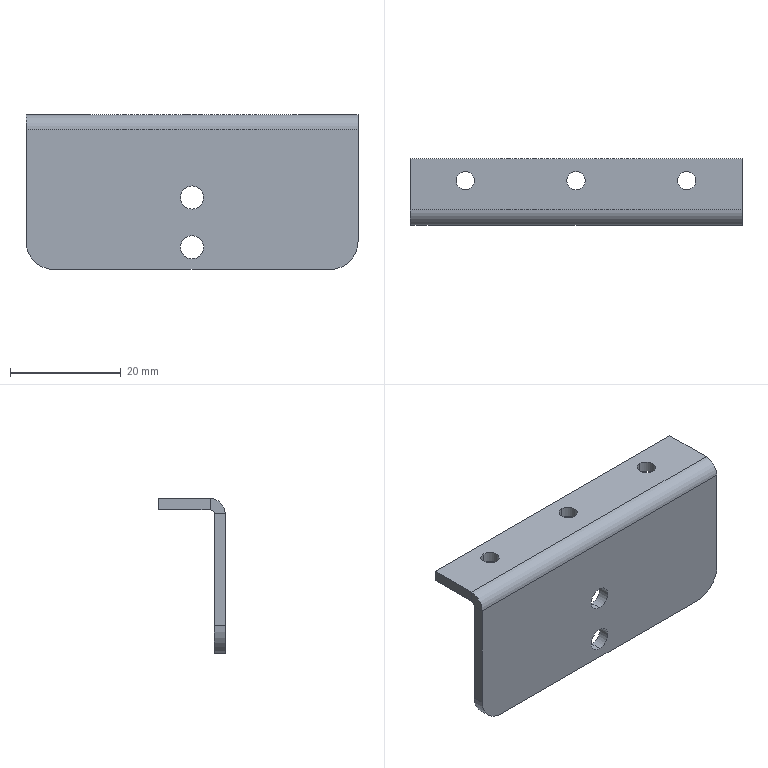Part | 1 solid | 26 faces | box 60 x 12 x 28 mm | volume 4342 mm3 | cylinder 14 | plane 12 | commonest cylinder face diameters 3.3 x6 4.2 x4 10 x2 1.48 x1 5.48 x1
STEP:
#1=CARTESIAN_POINT('',(20.,4.35,15.));
#2=VERTEX_POINT('',#1);
#3=CARTESIAN_POINT('',(20.,7.65,15.));
#4=VERTEX_POINT('',#3);
#5=CARTESIAN_POINT('',(20.,6.,15.));
#6=DIRECTION('',(0.,0.,-1.));
#7=DIRECTION('',(0.,1.,0.));
#8=AXIS2_PLACEMENT_3D('',#5,#6,#7);
#9=CIRCLE('',#8,1.65);
#10=EDGE_CURVE('',#2,#4,#9,.T.);
#11=ORIENTED_EDGE('',*,*,#10,.F.);
#12=CARTESIAN_POINT('',(20.,4.35,13.));
#13=VERTEX_POINT('',#12);
#14=CARTESIAN_POINT('',(20.,4.35,13.));
#15=DIRECTION('',(0.,0.,-1.));
#16=VECTOR('',#15,1000.);
#17=LINE('',#14,#16);
#18=EDGE_CURVE('',#2,#13,#17,.T.);
#19=ORIENTED_EDGE('',*,*,#18,.T.);
#20=CARTESIAN_POINT('',(20.,7.65,13.));
#21=VERTEX_POINT('',#20);
#22=CARTESIAN_POINT('',(20.,6.,13.));
#23=DIRECTION('',(0.,0.,-1.));
#24=DIRECTION('',(0.,1.,0.));
#25=AXIS2_PLACEMENT_3D('',#22,#23,#24);
#26=CIRCLE('',#25,1.65);
#27=EDGE_CURVE('',#13,#21,#26,.T.);
#28=ORIENTED_EDGE('',*,*,#27,.T.);
#29=CARTESIAN_POINT('',(20.,7.65,13.));
#30=DIRECTION('',(0.,0.,-1.));
#31=VECTOR('',#30,1000.);
#32=LINE('',#29,#31);
#33=EDGE_CURVE('',#4,#21,#32,.T.);
#34=ORIENTED_EDGE('',*,*,#33,.F.);
#35=EDGE_LOOP('',(#11,#19,#28,#34));
#36=FACE_OUTER_BOUND('',#35,.T.);
#37=CARTESIAN_POINT('',(20.,6.,13.));
#38=DIRECTION('',(0.,0.,-1.));
#39=DIRECTION('',(0.,1.,0.));
#40=AXIS2_PLACEMENT_3D('',#37,#38,#39);
#41=CYLINDRICAL_SURFACE('',#40,1.65);
#42=ADVANCED_FACE('',(#36),#41,.F.);
#43=CARTESIAN_POINT('',(-20.,4.35,15.));
#44=VERTEX_POINT('',#43);
#45=CARTESIAN_POINT('',(-20.,7.65,15.));
#46=VERTEX_POINT('',#45);
#47=CARTESIAN_POINT('',(-20.,6.,15.));
#48=DIRECTION('',(0.,0.,-1.));
#49=DIRECTION('',(0.,1.,0.));
#50=AXIS2_PLACEMENT_3D('',#47,#48,#49);
#51=CIRCLE('',#50,1.65);
#52=EDGE_CURVE('',#44,#46,#51,.T.);
#53=ORIENTED_EDGE('',*,*,#52,.F.);
#54=CARTESIAN_POINT('',(-20.,4.35,13.));
#55=VERTEX_POINT('',#54);
#56=CARTESIAN_POINT('',(-20.,4.35,13.));
#57=DIRECTION('',(0.,0.,-1.));
#58=VECTOR('',#57,1000.);
#59=LINE('',#56,#58);
#60=EDGE_CURVE('',#44,#55,#59,.T.);
#61=ORIENTED_EDGE('',*,*,#60,.T.);
#62=CARTESIAN_POINT('',(-20.,7.65,13.));
#63=VERTEX_POINT('',#62);
#64=CARTESIAN_POINT('',(-20.,6.,13.));
#65=DIRECTION('',(0.,0.,-1.));
#66=DIRECTION('',(0.,1.,0.));
#67=AXIS2_PLACEMENT_3D('',#64,#65,#66);
#68=CIRCLE('',#67,1.65);
#69=EDGE_CURVE('',#55,#63,#68,.T.);
#70=ORIENTED_EDGE('',*,*,#69,.T.);
#71=CARTESIAN_POINT('',(-20.,7.65,13.));
#72=DIRECTION('',(0.,0.,-1.));
#73=VECTOR('',#72,1000.);
#74=LINE('',#71,#73);
#75=EDGE_CURVE('',#46,#63,#74,.T.);
#76=ORIENTED_EDGE('',*,*,#75,.F.);
#77=EDGE_LOOP('',(#53,#61,#70,#76));
#78=FACE_OUTER_BOUND('',#77,.T.);
#79=CARTESIAN_POINT('',(-20.,6.,13.));
#80=DIRECTION('',(0.,0.,-1.));
#81=DIRECTION('',(0.,1.,0.));
#82=AXIS2_PLACEMENT_3D('',#79,#80,#81);
#83=CYLINDRICAL_SURFACE('',#82,1.65);
#84=ADVANCED_FACE('',(#78),#83,.F.);
#85=CARTESIAN_POINT('',(0.,4.35,15.));
#86=VERTEX_POINT('',#85);
#87=CARTESIAN_POINT('',(0.,7.65,15.));
#88=VERTEX_POINT('',#87);
#89=CARTESIAN_POINT('',(0.,6.,15.));
#90=DIRECTION('',(0.,0.,-1.));
#91=DIRECTION('',(0.,1.,0.));
#92=AXIS2_PLACEMENT_3D('',#89,#90,#91);
#93=CIRCLE('',#92,1.65);
#94=EDGE_CURVE('',#86,#88,#93,.T.);
#95=ORIENTED_EDGE('',*,*,#94,.F.);
#96=CARTESIAN_POINT('',(0.,4.35,13.));
#97=VERTEX_POINT('',#96);
#98=CARTESIAN_POINT('',(0.,4.35,13.));
#99=DIRECTION('',(0.,0.,-1.));
#100=VECTOR('',#99,1000.);
#101=LINE('',#98,#100);
#102=EDGE_CURVE('',#86,#97,#101,.T.);
#103=ORIENTED_EDGE('',*,*,#102,.T.);
#104=CARTESIAN_POINT('',(0.,7.65,13.));
#105=VERTEX_POINT('',#104);
#106=CARTESIAN_POINT('',(0.,6.,13.));
#107=DIRECTION('',(0.,0.,-1.));
#108=DIRECTION('',(0.,1.,0.));
#109=AXIS2_PLACEMENT_3D('',#106,#107,#108);
#110=CIRCLE('',#109,1.65);
#111=EDGE_CURVE('',#97,#105,#110,.T.);
#112=ORIENTED_EDGE('',*,*,#111,.T.);
#113=CARTESIAN_POINT('',(0.,7.65,13.));
#114=DIRECTION('',(0.,0.,-1.));
#115=VECTOR('',#114,1000.);
#116=LINE('',#113,#115);
#117=EDGE_CURVE('',#88,#105,#116,.T.);
#118=ORIENTED_EDGE('',*,*,#117,.F.);
#119=EDGE_LOOP('',(#95,#103,#112,#118));
#120=FACE_OUTER_BOUND('',#119,.T.);
#121=CARTESIAN_POINT('',(0.,6.,13.));
#122=DIRECTION('',(0.,0.,-1.));
#123=DIRECTION('',(0.,1.,0.));
#124=AXIS2_PLACEMENT_3D('',#121,#122,#123);
#125=CYLINDRICAL_SURFACE('',#124,1.65);
#126=ADVANCED_FACE('',(#120),#125,.F.);
#127=CARTESIAN_POINT('',(0.,-2.,-6.9));
#128=VERTEX_POINT('',#127);
#129=CARTESIAN_POINT('',(0.,-2.,-11.1));
#130=VERTEX_POINT('',#129);
#131=CARTESIAN_POINT('',(0.,-2.,-9.));
#132=DIRECTION('',(0.,-1.,0.));
#133=DIRECTION('',(0.,0.,-1.));
#134=AXIS2_PLACEMENT_3D('',#131,#132,#133);
#135=CIRCLE('',#134,2.1);
#136=EDGE_CURVE('',#128,#130,#135,.T.);
#137=ORIENTED_EDGE('',*,*,#136,.T.);
#138=CARTESIAN_POINT('',(0.,0.,-11.1));
#139=VERTEX_POINT('',#138);
#140=CARTESIAN_POINT('',(0.,-10.,-11.1));
#141=DIRECTION('',(0.,1.,0.));
#142=VECTOR('',#141,1000.);
#143=LINE('',#140,#142);
#144=EDGE_CURVE('',#130,#139,#143,.T.);
#145=ORIENTED_EDGE('',*,*,#144,.T.);
#146=CARTESIAN_POINT('',(0.,0.,-6.9));
#147=VERTEX_POINT('',#146);
#148=CARTESIAN_POINT('',(0.,0.,-9.));
#149=DIRECTION('',(0.,1.,0.));
#150=DIRECTION('',(0.,0.,1.));
#151=AXIS2_PLACEMENT_3D('',#148,#149,#150);
#152=CIRCLE('',#151,2.1);
#153=EDGE_CURVE('',#139,#147,#152,.T.);
#154=ORIENTED_EDGE('',*,*,#153,.T.);
#155=CARTESIAN_POINT('',(0.,-10.,-6.9));
#156=DIRECTION('',(0.,1.,0.));
#157=VECTOR('',#156,1000.);
#158=LINE('',#155,#157);
#159=EDGE_CURVE('',#128,#147,#158,.T.);
#160=ORIENTED_EDGE('',*,*,#159,.F.);
#161=EDGE_LOOP('',(#137,#145,#154,#160));
#162=FACE_OUTER_BOUND('',#161,.T.);
#163=CARTESIAN_POINT('',(0.,-10.,-9.));
#164=DIRECTION('',(0.,1.,0.));
#165=DIRECTION('',(0.,0.,1.));
#166=AXIS2_PLACEMENT_3D('',#163,#164,#165);
#167=CYLINDRICAL_SURFACE('',#166,2.1);
#168=ADVANCED_FACE('',(#162),#167,.F.);
#169=CARTESIAN_POINT('',(0.,-2.,2.1));
#170=VERTEX_POINT('',#169);
#171=CARTESIAN_POINT('',(0.,-2.,-2.1));
#172=VERTEX_POINT('',#171);
#173=CARTESIAN_POINT('',(0.,-2.,0.));
#174=DIRECTION('',(0.,-1.,0.));
#175=DIRECTION('',(0.,0.,-1.));
#176=AXIS2_PLACEMENT_3D('',#173,#174,#175);
#177=CIRCLE('',#176,2.1);
#178=EDGE_CURVE('',#170,#172,#177,.T.);
#179=ORIENTED_EDGE('',*,*,#178,.T.);
#180=CARTESIAN_POINT('',(0.,0.,-2.1));
#181=VERTEX_POINT('',#180);
#182=CARTESIAN_POINT('',(0.,-10.,-2.1));
#183=DIRECTION('',(0.,1.,0.));
#184=VECTOR('',#183,1000.);
#185=LINE('',#182,#184);
#186=EDGE_CURVE('',#172,#181,#185,.T.);
#187=ORIENTED_EDGE('',*,*,#186,.T.);
#188=CARTESIAN_POINT('',(0.,0.,2.1));
#189=VERTEX_POINT('',#188);
#190=CARTESIAN_POINT('',(0.,0.,0.));
#191=DIRECTION('',(0.,1.,0.));
#192=DIRECTION('',(0.,0.,1.));
#193=AXIS2_PLACEMENT_3D('',#190,#191,#192);
#194=CIRCLE('',#193,2.1);
#195=EDGE_CURVE('',#181,#189,#194,.T.);
#196=ORIENTED_EDGE('',*,*,#195,.T.);
#197=CARTESIAN_POINT('',(0.,-10.,2.1));
#198=DIRECTION('',(0.,1.,0.));
#199=VECTOR('',#198,1000.);
#200=LINE('',#197,#199);
#201=EDGE_CURVE('',#170,#189,#200,.T.);
#202=ORIENTED_EDGE('',*,*,#201,.F.);
#203=EDGE_LOOP('',(#179,#187,#196,#202));
#204=FACE_OUTER_BOUND('',#203,.T.);
#205=CARTESIAN_POINT('',(0.,-10.,0.));
#206=DIRECTION('',(0.,1.,0.));
#207=DIRECTION('',(0.,0.,1.));
#208=AXIS2_PLACEMENT_3D('',#205,#206,#207);
#209=CYLINDRICAL_SURFACE('',#208,2.1);
#210=ADVANCED_FACE('',(#204),#209,.F.);
#211=CARTESIAN_POINT('',(30.,-2.,12.26));
#212=VERTEX_POINT('',#211);
#213=CARTESIAN_POINT('',(30.,-2.,-8.));
#214=VERTEX_POINT('',#213);
#215=CARTESIAN_POINT('',(30.,-2.,15.));
#216=DIRECTION('',(0.,0.,-1.));
#217=VECTOR('',#216,1000.);
#218=LINE('',#215,#217);
#219=EDGE_CURVE('',#212,#214,#218,.T.);
#220=ORIENTED_EDGE('',*,*,#219,.T.);
#221=CARTESIAN_POINT('',(30.,0.,-8.));
#222=VERTEX_POINT('',#221);
#223=CARTESIAN_POINT('',(30.,-2.,-8.));
#224=DIRECTION('',(0.,1.,0.));
#225=VECTOR('',#224,1000.);
#226=LINE('',#223,#225);
#227=EDGE_CURVE('',#214,#222,#226,.T.);
#228=ORIENTED_EDGE('',*,*,#227,.T.);
#229=CARTESIAN_POINT('',(30.,0.,12.26));
#230=VERTEX_POINT('',#229);
#231=CARTESIAN_POINT('',(30.,0.,15.));
#232=DIRECTION('',(0.,0.,-1.));
#233=VECTOR('',#232,1000.);
#234=LINE('',#231,#233);
#235=EDGE_CURVE('',#230,#222,#234,.T.);
#236=ORIENTED_EDGE('',*,*,#235,.F.);
#237=CARTESIAN_POINT('',(30.,0.,12.26));
#238=DIRECTION('',(0.,-1.,0.));
#239=VECTOR('',#238,1000.);
#240=LINE('',#237,#239);
#241=EDGE_CURVE('',#230,#212,#240,.T.);
#242=ORIENTED_EDGE('',*,*,#241,.T.);
#243=EDGE_LOOP('',(#220,#228,#236,#242));
#244=FACE_OUTER_BOUND('',#243,.T.);
#245=CARTESIAN_POINT('',(30.,-2.,15.));
#246=DIRECTION('',(1.,0.,0.));
#247=DIRECTION('',(0.,0.,-1.));
#248=AXIS2_PLACEMENT_3D('',#245,#246,#247);
#249=PLANE('',#248);
#250=ADVANCED_FACE('',(#244),#249,.T.);
#251=ORIENTED_EDGE('',*,*,#136,.F.);
#252=CARTESIAN_POINT('',(0.,-2.,-9.));
#253=DIRECTION('',(0.,-1.,0.));
#254=DIRECTION('',(0.,0.,-1.));
#255=AXIS2_PLACEMENT_3D('',#252,#253,#254);
#256=CIRCLE('',#255,2.1);
#257=EDGE_CURVE('',#130,#128,#256,.T.);
#258=ORIENTED_EDGE('',*,*,#257,.F.);
#259=EDGE_LOOP('',(#251,#258));
#260=FACE_BOUND('',#259,.T.);
#261=ORIENTED_EDGE('',*,*,#178,.F.);
#262=CARTESIAN_POINT('',(0.,-2.,0.));
#263=DIRECTION('',(0.,-1.,0.));
#264=DIRECTION('',(0.,0.,-1.));
#265=AXIS2_PLACEMENT_3D('',#262,#263,#264);
#266=CIRCLE('',#265,2.1);
#267=EDGE_CURVE('',#172,#170,#266,.T.);
#268=ORIENTED_EDGE('',*,*,#267,.F.);
#269=EDGE_LOOP('',(#261,#268));
#270=FACE_BOUND('',#269,.T.);
#271=CARTESIAN_POINT('',(25.,-2.,-13.));
#272=VERTEX_POINT('',#271);
#273=CARTESIAN_POINT('',(-25.,-2.,-13.));
#274=VERTEX_POINT('',#273);
#275=CARTESIAN_POINT('',(-30.,-2.,-13.));
#276=DIRECTION('',(-1.,0.,0.));
#277=VECTOR('',#276,1000.);
#278=LINE('',#275,#277);
#279=EDGE_CURVE('',#272,#274,#278,.T.);
#280=ORIENTED_EDGE('',*,*,#279,.F.);
#281=CARTESIAN_POINT('',(25.,-2.,-8.));
#282=DIRECTION('',(0.,-1.,0.));
#283=DIRECTION('',(0.,0.,-1.));
#284=AXIS2_PLACEMENT_3D('',#281,#282,#283);
#285=CIRCLE('',#284,5.);
#286=EDGE_CURVE('',#272,#214,#285,.T.);
#287=ORIENTED_EDGE('',*,*,#286,.T.);
#288=ORIENTED_EDGE('',*,*,#219,.F.);
#289=CARTESIAN_POINT('',(-30.,-2.,12.26));
#290=VERTEX_POINT('',#289);
#291=CARTESIAN_POINT('',(30.,-2.,12.26));
#292=DIRECTION('',(-1.,0.,0.));
#293=VECTOR('',#292,1000.);
#294=LINE('',#291,#293);
#295=EDGE_CURVE('',#212,#290,#294,.T.);
#296=ORIENTED_EDGE('',*,*,#295,.T.);
#297=CARTESIAN_POINT('',(-30.,-2.,-8.));
#298=VERTEX_POINT('',#297);
#299=CARTESIAN_POINT('',(-30.,-2.,15.));
#300=DIRECTION('',(0.,0.,1.));
#301=VECTOR('',#300,1000.);
#302=LINE('',#299,#301);
#303=EDGE_CURVE('',#298,#290,#302,.T.);
#304=ORIENTED_EDGE('',*,*,#303,.F.);
#305=CARTESIAN_POINT('',(-25.,-2.,-8.));
#306=DIRECTION('',(0.,-1.,0.));
#307=DIRECTION('',(0.,0.,-1.));
#308=AXIS2_PLACEMENT_3D('',#305,#306,#307);
#309=CIRCLE('',#308,5.);
#310=EDGE_CURVE('',#298,#274,#309,.T.);
#311=ORIENTED_EDGE('',*,*,#310,.T.);
#312=EDGE_LOOP('',(#280,#287,#288,#296,#304,#311));
#313=FACE_OUTER_BOUND('',#312,.T.);
#314=CARTESIAN_POINT('',(0.,-2.,0.));
#315=DIRECTION('',(0.,-1.,0.));
#316=DIRECTION('',(0.,0.,-1.));
#317=AXIS2_PLACEMENT_3D('',#314,#315,#316);
#318=PLANE('',#317);
#319=ADVANCED_FACE('',(#260,#270,#313),#318,.T.);
#320=CARTESIAN_POINT('',(0.,0.,0.));
#321=DIRECTION('',(0.,1.,0.));
#322=DIRECTION('',(0.,0.,1.));
#323=AXIS2_PLACEMENT_3D('',#320,#321,#322);
#324=CIRCLE('',#323,2.1);
#325=EDGE_CURVE('',#189,#181,#324,.T.);
#326=ORIENTED_EDGE('',*,*,#325,.F.);
#327=ORIENTED_EDGE('',*,*,#195,.F.);
#328=EDGE_LOOP('',(#326,#327));
#329=FACE_BOUND('',#328,.T.);
#330=CARTESIAN_POINT('',(0.,0.,-9.));
#331=DIRECTION('',(0.,1.,0.));
#332=DIRECTION('',(0.,0.,1.));
#333=AXIS2_PLACEMENT_3D('',#330,#331,#332);
#334=CIRCLE('',#333,2.1);
#335=EDGE_CURVE('',#147,#139,#334,.T.);
#336=ORIENTED_EDGE('',*,*,#335,.F.);
#337=ORIENTED_EDGE('',*,*,#153,.F.);
#338=EDGE_LOOP('',(#336,#337));
#339=FACE_BOUND('',#338,.T.);
#340=ORIENTED_EDGE('',*,*,#235,.T.);
#341=CARTESIAN_POINT('',(25.,0.,-13.));
#342=VERTEX_POINT('',#341);
#343=CARTESIAN_POINT('',(25.,0.,-8.));
#344=DIRECTION('',(0.,1.,0.));
#345=DIRECTION('',(0.,0.,-1.));
#346=AXIS2_PLACEMENT_3D('',#343,#344,#345);
#347=CIRCLE('',#346,5.);
#348=EDGE_CURVE('',#222,#342,#347,.T.);
#349=ORIENTED_EDGE('',*,*,#348,.T.);
#350=CARTESIAN_POINT('',(-25.,0.,-13.));
#351=VERTEX_POINT('',#350);
#352=CARTESIAN_POINT('',(-30.,0.,-13.));
#353=DIRECTION('',(-1.,0.,0.));
#354=VECTOR('',#353,1000.);
#355=LINE('',#352,#354);
#356=EDGE_CURVE('',#342,#351,#355,.T.);
#357=ORIENTED_EDGE('',*,*,#356,.T.);
#358=CARTESIAN_POINT('',(-30.,0.,-8.));
#359=VERTEX_POINT('',#358);
#360=CARTESIAN_POINT('',(-25.,0.,-8.));
#361=DIRECTION('',(0.,1.,0.));
#362=DIRECTION('',(0.,0.,-1.));
#363=AXIS2_PLACEMENT_3D('',#360,#361,#362);
#364=CIRCLE('',#363,5.);
#365=EDGE_CURVE('',#351,#359,#364,.T.);
#366=ORIENTED_EDGE('',*,*,#365,.T.);
#367=CARTESIAN_POINT('',(-30.,0.,12.26));
#368=VERTEX_POINT('',#367);
#369=CARTESIAN_POINT('',(-30.,0.,15.));
#370=DIRECTION('',(0.,0.,1.));
#371=VECTOR('',#370,1000.);
#372=LINE('',#369,#371);
#373=EDGE_CURVE('',#359,#368,#372,.T.);
#374=ORIENTED_EDGE('',*,*,#373,.T.);
#375=CARTESIAN_POINT('',(30.,0.,12.26));
#376=DIRECTION('',(-1.,0.,0.));
#377=VECTOR('',#376,1000.);
#378=LINE('',#375,#377);
#379=EDGE_CURVE('',#230,#368,#378,.T.);
#380=ORIENTED_EDGE('',*,*,#379,.F.);
#381=EDGE_LOOP('',(#340,#349,#357,#366,#374,#380));
#382=FACE_OUTER_BOUND('',#381,.T.);
#383=CARTESIAN_POINT('',(0.,0.,0.));
#384=DIRECTION('',(0.,-1.,0.));
#385=DIRECTION('',(0.,0.,-1.));
#386=AXIS2_PLACEMENT_3D('',#383,#384,#385);
#387=PLANE('',#386);
#388=ADVANCED_FACE('',(#329,#339,#382),#387,.F.);
#389=ORIENTED_EDGE('',*,*,#373,.F.);
#390=CARTESIAN_POINT('',(-30.,-2.,-8.));
#391=DIRECTION('',(0.,-1.,0.));
#392=VECTOR('',#391,1000.);
#393=LINE('',#390,#392);
#394=EDGE_CURVE('',#359,#298,#393,.T.);
#395=ORIENTED_EDGE('',*,*,#394,.T.);
#396=ORIENTED_EDGE('',*,*,#303,.T.);
#397=CARTESIAN_POINT('',(-30.,0.,12.26));
#398=DIRECTION('',(0.,-1.,0.));
#399=VECTOR('',#398,1000.);
#400=LINE('',#397,#399);
#401=EDGE_CURVE('',#368,#290,#400,.T.);
#402=ORIENTED_EDGE('',*,*,#401,.F.);
#403=EDGE_LOOP('',(#389,#395,#396,#402));
#404=FACE_OUTER_BOUND('',#403,.T.);
#405=CARTESIAN_POINT('',(-30.,-2.,15.));
#406=DIRECTION('',(-1.,0.,0.));
#407=DIRECTION('',(0.,0.,1.));
#408=AXIS2_PLACEMENT_3D('',#405,#406,#407);
#409=PLANE('',#408);
#410=ADVANCED_FACE('',(#404),#409,.T.);
#411=ORIENTED_EDGE('',*,*,#356,.F.);
#412=CARTESIAN_POINT('',(25.,-2.,-13.));
#413=DIRECTION('',(0.,-1.,0.));
#414=VECTOR('',#413,1000.);
#415=LINE('',#412,#414);
#416=EDGE_CURVE('',#342,#272,#415,.T.);
#417=ORIENTED_EDGE('',*,*,#416,.T.);
#418=ORIENTED_EDGE('',*,*,#279,.T.);
#419=CARTESIAN_POINT('',(-25.,-2.,-13.));
#420=DIRECTION('',(0.,1.,0.));
#421=VECTOR('',#420,1000.);
#422=LINE('',#419,#421);
#423=EDGE_CURVE('',#274,#351,#422,.T.);
#424=ORIENTED_EDGE('',*,*,#423,.T.);
#425=EDGE_LOOP('',(#411,#417,#418,#424));
#426=FACE_OUTER_BOUND('',#425,.T.);
#427=CARTESIAN_POINT('',(-30.,-2.,-13.));
#428=DIRECTION('',(0.,0.,-1.));
#429=DIRECTION('',(-1.,0.,0.));
#430=AXIS2_PLACEMENT_3D('',#427,#428,#429);
#431=PLANE('',#430);
#432=ADVANCED_FACE('',(#426),#431,.T.);
#433=ORIENTED_EDGE('',*,*,#186,.F.);
#434=ORIENTED_EDGE('',*,*,#267,.T.);
#435=ORIENTED_EDGE('',*,*,#201,.T.);
#436=ORIENTED_EDGE('',*,*,#325,.T.);
#437=EDGE_LOOP('',(#433,#434,#435,#436));
#438=FACE_OUTER_BOUND('',#437,.T.);
#439=CARTESIAN_POINT('',(0.,-10.,0.));
#440=DIRECTION('',(0.,1.,0.));
#441=DIRECTION('',(0.,0.,1.));
#442=AXIS2_PLACEMENT_3D('',#439,#440,#441);
#443=CYLINDRICAL_SURFACE('',#442,2.1);
#444=ADVANCED_FACE('',(#438),#443,.F.);
#445=ORIENTED_EDGE('',*,*,#144,.F.);
#446=ORIENTED_EDGE('',*,*,#257,.T.);
#447=ORIENTED_EDGE('',*,*,#159,.T.);
#448=ORIENTED_EDGE('',*,*,#335,.T.);
#449=EDGE_LOOP('',(#445,#446,#447,#448));
#450=FACE_OUTER_BOUND('',#449,.T.);
#451=CARTESIAN_POINT('',(0.,-10.,-9.));
#452=DIRECTION('',(0.,1.,0.));
#453=DIRECTION('',(0.,0.,1.));
#454=AXIS2_PLACEMENT_3D('',#451,#452,#453);
#455=CYLINDRICAL_SURFACE('',#454,2.1);
#456=ADVANCED_FACE('',(#450),#455,.F.);
#457=CARTESIAN_POINT('',(-30.,0.74,13.));
#458=VERTEX_POINT('',#457);
#459=CARTESIAN_POINT('',(-30.,0.74,15.));
#460=VERTEX_POINT('',#459);
#461=CARTESIAN_POINT('',(-30.,0.74,15.));
#462=DIRECTION('',(0.,0.,1.));
#463=VECTOR('',#462,1000.);
#464=LINE('',#461,#463);
#465=EDGE_CURVE('',#458,#460,#464,.T.);
#466=ORIENTED_EDGE('',*,*,#465,.F.);
#467=CARTESIAN_POINT('',(-30.,0.74,12.26));
#468=DIRECTION('',(-1.,0.,0.));
#469=DIRECTION('',(0.,0.,-1.));
#470=AXIS2_PLACEMENT_3D('',#467,#468,#469);
#471=CIRCLE('',#470,0.74);
#472=EDGE_CURVE('',#368,#458,#471,.T.);
#473=ORIENTED_EDGE('',*,*,#472,.F.);
#474=ORIENTED_EDGE('',*,*,#401,.T.);
#475=CARTESIAN_POINT('',(-30.,0.74,12.26));
#476=DIRECTION('',(-1.,0.,0.));
#477=DIRECTION('',(0.,0.,-1.));
#478=AXIS2_PLACEMENT_3D('',#475,#476,#477);
#479=CIRCLE('',#478,2.74);
#480=EDGE_CURVE('',#290,#460,#479,.T.);
#481=ORIENTED_EDGE('',*,*,#480,.T.);
#482=EDGE_LOOP('',(#466,#473,#474,#481));
#483=FACE_OUTER_BOUND('',#482,.T.);
#484=CARTESIAN_POINT('',(-30.,0.74,12.26));
#485=DIRECTION('',(-1.,0.,0.));
#486=DIRECTION('',(0.,0.,1.));
#487=AXIS2_PLACEMENT_3D('',#484,#485,#486);
#488=PLANE('',#487);
#489=ADVANCED_FACE('',(#483),#488,.T.);
#490=CARTESIAN_POINT('',(30.,0.74,13.));
#491=VERTEX_POINT('',#490);
#492=CARTESIAN_POINT('',(30.,0.74,12.26));
#493=DIRECTION('',(1.,0.,0.));
#494=DIRECTION('',(0.,0.,-1.));
#495=AXIS2_PLACEMENT_3D('',#492,#493,#494);
#496=CIRCLE('',#495,0.74);
#497=EDGE_CURVE('',#491,#230,#496,.T.);
#498=ORIENTED_EDGE('',*,*,#497,.F.);
#499=CARTESIAN_POINT('',(30.,0.74,15.));
#500=VERTEX_POINT('',#499);
#501=CARTESIAN_POINT('',(30.,0.74,13.));
#502=DIRECTION('',(0.,0.,1.));
#503=VECTOR('',#502,1000.);
#504=LINE('',#501,#503);
#505=EDGE_CURVE('',#491,#500,#504,.T.);
#506=ORIENTED_EDGE('',*,*,#505,.T.);
#507=CARTESIAN_POINT('',(30.,0.74,12.26));
#508=DIRECTION('',(1.,0.,0.));
#509=DIRECTION('',(0.,0.,-1.));
#510=AXIS2_PLACEMENT_3D('',#507,#508,#509);
#511=CIRCLE('',#510,2.74);
#512=EDGE_CURVE('',#500,#212,#511,.T.);
#513=ORIENTED_EDGE('',*,*,#512,.T.);
#514=ORIENTED_EDGE('',*,*,#241,.F.);
#515=EDGE_LOOP('',(#498,#506,#513,#514));
#516=FACE_OUTER_BOUND('',#515,.T.);
#517=CARTESIAN_POINT('',(30.,0.74,12.26));
#518=DIRECTION('',(-1.,0.,0.));
#519=DIRECTION('',(0.,0.,1.));
#520=AXIS2_PLACEMENT_3D('',#517,#518,#519);
#521=PLANE('',#520);
#522=ADVANCED_FACE('',(#516),#521,.F.);
#523=ORIENTED_EDGE('',*,*,#295,.F.);
#524=ORIENTED_EDGE('',*,*,#512,.F.);
#525=CARTESIAN_POINT('',(0.,0.74,15.));
#526=DIRECTION('',(1.,0.,0.));
#527=VECTOR('',#526,1000.);
#528=LINE('',#525,#527);
#529=EDGE_CURVE('',#460,#500,#528,.T.);
#530=ORIENTED_EDGE('',*,*,#529,.F.);
#531=ORIENTED_EDGE('',*,*,#480,.F.);
#532=EDGE_LOOP('',(#523,#524,#530,#531));
#533=FACE_OUTER_BOUND('',#532,.T.);
#534=CARTESIAN_POINT('',(30.,0.74,12.26));
#535=DIRECTION('',(1.,0.,0.));
#536=DIRECTION('',(0.,0.,1.));
#537=AXIS2_PLACEMENT_3D('',#534,#535,#536);
#538=CYLINDRICAL_SURFACE('',#537,2.74);
#539=ADVANCED_FACE('',(#533),#538,.T.);
#540=ORIENTED_EDGE('',*,*,#379,.T.);
#541=ORIENTED_EDGE('',*,*,#472,.T.);
#542=CARTESIAN_POINT('',(-30.,0.74,13.));
#543=DIRECTION('',(1.,0.,0.));
#544=VECTOR('',#543,1000.);
#545=LINE('',#542,#544);
#546=EDGE_CURVE('',#458,#491,#545,.T.);
#547=ORIENTED_EDGE('',*,*,#546,.T.);
#548=ORIENTED_EDGE('',*,*,#497,.T.);
#549=EDGE_LOOP('',(#540,#541,#547,#548));
#550=FACE_OUTER_BOUND('',#549,.T.);
#551=CARTESIAN_POINT('',(30.,0.74,12.26));
#552=DIRECTION('',(1.,0.,0.));
#553=DIRECTION('',(0.,0.,1.));
#554=AXIS2_PLACEMENT_3D('',#551,#552,#553);
#555=CYLINDRICAL_SURFACE('',#554,0.74);
#556=ADVANCED_FACE('',(#550),#555,.F.);
#557=CARTESIAN_POINT('',(30.,10.,15.));
#558=VERTEX_POINT('',#557);
#559=CARTESIAN_POINT('',(30.,0.,15.));
#560=DIRECTION('',(0.,-1.,0.));
#561=VECTOR('',#560,1000.);
#562=LINE('',#559,#561);
#563=EDGE_CURVE('',#558,#500,#562,.T.);
#564=ORIENTED_EDGE('',*,*,#563,.T.);
#565=ORIENTED_EDGE('',*,*,#505,.F.);
#566=CARTESIAN_POINT('',(30.,10.,13.));
#567=VERTEX_POINT('',#566);
#568=CARTESIAN_POINT('',(30.,0.,13.));
#569=DIRECTION('',(0.,-1.,0.));
#570=VECTOR('',#569,1000.);
#571=LINE('',#568,#570);
#572=EDGE_CURVE('',#567,#491,#571,.T.);
#573=ORIENTED_EDGE('',*,*,#572,.F.);
#574=CARTESIAN_POINT('',(30.,10.,15.));
#575=DIRECTION('',(0.,0.,-1.));
#576=VECTOR('',#575,1000.);
#577=LINE('',#574,#576);
#578=EDGE_CURVE('',#558,#567,#577,.T.);
#579=ORIENTED_EDGE('',*,*,#578,.F.);
#580=EDGE_LOOP('',(#564,#565,#573,#579));
#581=FACE_OUTER_BOUND('',#580,.T.);
#582=CARTESIAN_POINT('',(30.,0.,15.));
#583=DIRECTION('',(1.,0.,0.));
#584=DIRECTION('',(0.,0.,-1.));
#585=AXIS2_PLACEMENT_3D('',#582,#583,#584);
#586=PLANE('',#585);
#587=ADVANCED_FACE('',(#581),#586,.T.);
#588=CARTESIAN_POINT('',(-30.,10.,13.));
#589=VERTEX_POINT('',#588);
#590=CARTESIAN_POINT('',(-30.,0.,13.));
#591=DIRECTION('',(0.,1.,0.));
#592=VECTOR('',#591,1000.);
#593=LINE('',#590,#592);
#594=EDGE_CURVE('',#458,#589,#593,.T.);
#595=ORIENTED_EDGE('',*,*,#594,.F.);
#596=ORIENTED_EDGE('',*,*,#465,.T.);
#597=CARTESIAN_POINT('',(-30.,10.,15.));
#598=VERTEX_POINT('',#597);
#599=CARTESIAN_POINT('',(-30.,10.,15.));
#600=DIRECTION('',(0.,1.,0.));
#601=VECTOR('',#600,1000.);
#602=LINE('',#599,#601);
#603=EDGE_CURVE('',#460,#598,#602,.T.);
#604=ORIENTED_EDGE('',*,*,#603,.T.);
#605=CARTESIAN_POINT('',(-30.,10.,15.));
#606=DIRECTION('',(0.,0.,-1.));
#607=VECTOR('',#606,1000.);
#608=LINE('',#605,#607);
#609=EDGE_CURVE('',#598,#589,#608,.T.);
#610=ORIENTED_EDGE('',*,*,#609,.T.);
#611=EDGE_LOOP('',(#595,#596,#604,#610));
#612=FACE_OUTER_BOUND('',#611,.T.);
#613=CARTESIAN_POINT('',(-30.,10.,15.));
#614=DIRECTION('',(-1.,0.,0.));
#615=DIRECTION('',(0.,0.,1.));
#616=AXIS2_PLACEMENT_3D('',#613,#614,#615);
#617=PLANE('',#616);
#618=ADVANCED_FACE('',(#612),#617,.T.);
#619=CARTESIAN_POINT('',(20.,6.,15.));
#620=DIRECTION('',(0.,0.,-1.));
#621=DIRECTION('',(0.,1.,0.));
#622=AXIS2_PLACEMENT_3D('',#619,#620,#621);
#623=CIRCLE('',#622,1.65);
#624=EDGE_CURVE('',#4,#2,#623,.T.);
#625=ORIENTED_EDGE('',*,*,#624,.T.);
#626=ORIENTED_EDGE('',*,*,#10,.T.);
#627=EDGE_LOOP('',(#625,#626));
#628=FACE_BOUND('',#627,.T.);
#629=CARTESIAN_POINT('',(-20.,6.,15.));
#630=DIRECTION('',(0.,0.,-1.));
#631=DIRECTION('',(0.,1.,0.));
#632=AXIS2_PLACEMENT_3D('',#629,#630,#631);
#633=CIRCLE('',#632,1.65);
#634=EDGE_CURVE('',#46,#44,#633,.T.);
#635=ORIENTED_EDGE('',*,*,#634,.T.);
#636=ORIENTED_EDGE('',*,*,#52,.T.);
#637=EDGE_LOOP('',(#635,#636));
#638=FACE_BOUND('',#637,.T.);
#639=CARTESIAN_POINT('',(0.,6.,15.));
#640=DIRECTION('',(0.,0.,-1.));
#641=DIRECTION('',(0.,1.,0.));
#642=AXIS2_PLACEMENT_3D('',#639,#640,#641);
#643=CIRCLE('',#642,1.65);
#644=EDGE_CURVE('',#88,#86,#643,.T.);
#645=ORIENTED_EDGE('',*,*,#644,.T.);
#646=ORIENTED_EDGE('',*,*,#94,.T.);
#647=EDGE_LOOP('',(#645,#646));
#648=FACE_BOUND('',#647,.T.);
#649=ORIENTED_EDGE('',*,*,#603,.F.);
#650=ORIENTED_EDGE('',*,*,#529,.T.);
#651=ORIENTED_EDGE('',*,*,#563,.F.);
#652=CARTESIAN_POINT('',(30.,10.,15.));
#653=DIRECTION('',(1.,0.,0.));
#654=VECTOR('',#653,1000.);
#655=LINE('',#652,#654);
#656=EDGE_CURVE('',#598,#558,#655,.T.);
#657=ORIENTED_EDGE('',*,*,#656,.F.);
#658=EDGE_LOOP('',(#649,#650,#651,#657));
#659=FACE_OUTER_BOUND('',#658,.T.);
#660=CARTESIAN_POINT('',(0.,0.,15.));
#661=DIRECTION('',(0.,0.,1.));
#662=DIRECTION('',(0.,-1.,0.));
#663=AXIS2_PLACEMENT_3D('',#660,#661,#662);
#664=PLANE('',#663);
#665=ADVANCED_FACE('',(#628,#638,#648,#659),#664,.T.);
#666=CARTESIAN_POINT('',(20.,6.,13.));
#667=DIRECTION('',(0.,0.,-1.));
#668=DIRECTION('',(0.,1.,0.));
#669=AXIS2_PLACEMENT_3D('',#666,#667,#668);
#670=CIRCLE('',#669,1.65);
#671=EDGE_CURVE('',#21,#13,#670,.T.);
#672=ORIENTED_EDGE('',*,*,#671,.F.);
#673=ORIENTED_EDGE('',*,*,#27,.F.);
#674=EDGE_LOOP('',(#672,#673));
#675=FACE_BOUND('',#674,.T.);
#676=CARTESIAN_POINT('',(-20.,6.,13.));
#677=DIRECTION('',(0.,0.,-1.));
#678=DIRECTION('',(0.,1.,0.));
#679=AXIS2_PLACEMENT_3D('',#676,#677,#678);
#680=CIRCLE('',#679,1.65);
#681=EDGE_CURVE('',#63,#55,#680,.T.);
#682=ORIENTED_EDGE('',*,*,#681,.F.);
#683=ORIENTED_EDGE('',*,*,#69,.F.);
#684=EDGE_LOOP('',(#682,#683));
#685=FACE_BOUND('',#684,.T.);
#686=CARTESIAN_POINT('',(0.,6.,13.));
#687=DIRECTION('',(0.,0.,-1.));
#688=DIRECTION('',(0.,1.,0.));
#689=AXIS2_PLACEMENT_3D('',#686,#687,#688);
#690=CIRCLE('',#689,1.65);
#691=EDGE_CURVE('',#105,#97,#690,.T.);
#692=ORIENTED_EDGE('',*,*,#691,.F.);
#693=ORIENTED_EDGE('',*,*,#111,.F.);
#694=EDGE_LOOP('',(#692,#693));
#695=FACE_BOUND('',#694,.T.);
#696=ORIENTED_EDGE('',*,*,#546,.F.);
#697=ORIENTED_EDGE('',*,*,#594,.T.);
#698=CARTESIAN_POINT('',(0.,10.,13.));
#699=DIRECTION('',(1.,0.,0.));
#700=VECTOR('',#699,1000.);
#701=LINE('',#698,#700);
#702=EDGE_CURVE('',#589,#567,#701,.T.);
#703=ORIENTED_EDGE('',*,*,#702,.T.);
#704=ORIENTED_EDGE('',*,*,#572,.T.);
#705=EDGE_LOOP('',(#696,#697,#703,#704));
#706=FACE_OUTER_BOUND('',#705,.T.);
#707=CARTESIAN_POINT('',(0.,0.,13.));
#708=DIRECTION('',(0.,0.,1.));
#709=DIRECTION('',(0.,-1.,0.));
#710=AXIS2_PLACEMENT_3D('',#707,#708,#709);
#711=PLANE('',#710);
#712=ADVANCED_FACE('',(#675,#685,#695,#706),#711,.F.);
#713=ORIENTED_EDGE('',*,*,#702,.F.);
#714=ORIENTED_EDGE('',*,*,#609,.F.);
#715=ORIENTED_EDGE('',*,*,#656,.T.);
#716=ORIENTED_EDGE('',*,*,#578,.T.);
#717=EDGE_LOOP('',(#713,#714,#715,#716));
#718=FACE_OUTER_BOUND('',#717,.T.);
#719=CARTESIAN_POINT('',(30.,10.,15.));
#720=DIRECTION('',(0.,1.,0.));
#721=DIRECTION('',(0.,0.,1.));
#722=AXIS2_PLACEMENT_3D('',#719,#720,#721);
#723=PLANE('',#722);
#724=ADVANCED_FACE('',(#718),#723,.T.);
#725=ORIENTED_EDGE('',*,*,#286,.F.);
#726=ORIENTED_EDGE('',*,*,#416,.F.);
#727=ORIENTED_EDGE('',*,*,#348,.F.);
#728=ORIENTED_EDGE('',*,*,#227,.F.);
#729=EDGE_LOOP('',(#725,#726,#727,#728));
#730=FACE_OUTER_BOUND('',#729,.T.);
#731=CARTESIAN_POINT('',(25.,-2.,-8.));
#732=DIRECTION('',(0.,1.,0.));
#733=DIRECTION('',(0.,0.,1.));
#734=AXIS2_PLACEMENT_3D('',#731,#732,#733);
#735=CYLINDRICAL_SURFACE('',#734,5.);
#736=ADVANCED_FACE('',(#730),#735,.T.);
#737=ORIENTED_EDGE('',*,*,#310,.F.);
#738=ORIENTED_EDGE('',*,*,#394,.F.);
#739=ORIENTED_EDGE('',*,*,#365,.F.);
#740=ORIENTED_EDGE('',*,*,#423,.F.);
#741=EDGE_LOOP('',(#737,#738,#739,#740));
#742=FACE_OUTER_BOUND('',#741,.T.);
#743=CARTESIAN_POINT('',(-25.,-2.,-8.));
#744=DIRECTION('',(0.,1.,0.));
#745=DIRECTION('',(0.,0.,1.));
#746=AXIS2_PLACEMENT_3D('',#743,#744,#745);
#747=CYLINDRICAL_SURFACE('',#746,5.);
#748=ADVANCED_FACE('',(#742),#747,.T.);
#749=ORIENTED_EDGE('',*,*,#102,.F.);
#750=ORIENTED_EDGE('',*,*,#644,.F.);
#751=ORIENTED_EDGE('',*,*,#117,.T.);
#752=ORIENTED_EDGE('',*,*,#691,.T.);
#753=EDGE_LOOP('',(#749,#750,#751,#752));
#754=FACE_OUTER_BOUND('',#753,.T.);
#755=CARTESIAN_POINT('',(0.,6.,13.));
#756=DIRECTION('',(0.,0.,-1.));
#757=DIRECTION('',(0.,1.,0.));
#758=AXIS2_PLACEMENT_3D('',#755,#756,#757);
#759=CYLINDRICAL_SURFACE('',#758,1.65);
#760=ADVANCED_FACE('',(#754),#759,.F.);
#761=ORIENTED_EDGE('',*,*,#60,.F.);
#762=ORIENTED_EDGE('',*,*,#634,.F.);
#763=ORIENTED_EDGE('',*,*,#75,.T.);
#764=ORIENTED_EDGE('',*,*,#681,.T.);
#765=EDGE_LOOP('',(#761,#762,#763,#764));
#766=FACE_OUTER_BOUND('',#765,.T.);
#767=CARTESIAN_POINT('',(-20.,6.,13.));
#768=DIRECTION('',(0.,0.,-1.));
#769=DIRECTION('',(0.,1.,0.));
#770=AXIS2_PLACEMENT_3D('',#767,#768,#769);
#771=CYLINDRICAL_SURFACE('',#770,1.65);
#772=ADVANCED_FACE('',(#766),#771,.F.);
#773=ORIENTED_EDGE('',*,*,#18,.F.);
#774=ORIENTED_EDGE('',*,*,#624,.F.);
#775=ORIENTED_EDGE('',*,*,#33,.T.);
#776=ORIENTED_EDGE('',*,*,#671,.T.);
#777=EDGE_LOOP('',(#773,#774,#775,#776));
#778=FACE_OUTER_BOUND('',#777,.T.);
#779=CARTESIAN_POINT('',(20.,6.,13.));
#780=DIRECTION('',(0.,0.,-1.));
#781=DIRECTION('',(0.,1.,0.));
#782=AXIS2_PLACEMENT_3D('',#779,#780,#781);
#783=CYLINDRICAL_SURFACE('',#782,1.65);
#784=ADVANCED_FACE('',(#778),#783,.F.);
#785=CLOSED_SHELL('',(#42,#84,#126,#168,#210,#250,#319,#388,#410,#432,#444,#456,#489,#522,#539,#556,#587,#618,#665,#712,#724,#736,#748,#760,#772,#784));
#786=MANIFOLD_SOLID_BREP('',#785);
#787=CARTESIAN_POINT('',(0.,0.,0.));
#788=DIRECTION('',(0.,0.,1.));
#789=DIRECTION('',(1.,0.,0.));
#790=AXIS2_PLACEMENT_3D('',#787,#788,#789);
#791=(LENGTH_UNIT()NAMED_UNIT(*)SI_UNIT(.MILLI.,.METRE.));
#792=UNCERTAINTY_MEASURE_WITH_UNIT(LENGTH_MEASURE(0.00001),#791,'','');
#793=(NAMED_UNIT(*)PLANE_ANGLE_UNIT()SI_UNIT($,.RADIAN.));
#794=(NAMED_UNIT(*)SI_UNIT($,.STERADIAN.)SOLID_ANGLE_UNIT());
#795=(GEOMETRIC_REPRESENTATION_CONTEXT(3)GLOBAL_UNCERTAINTY_ASSIGNED_CONTEXT((#792))GLOBAL_UNIT_ASSIGNED_CONTEXT((#791,#793,#794))REPRESENTATION_CONTEXT('',''));
#796=ADVANCED_BREP_SHAPE_REPRESENTATION('',(#786,#790),#795);